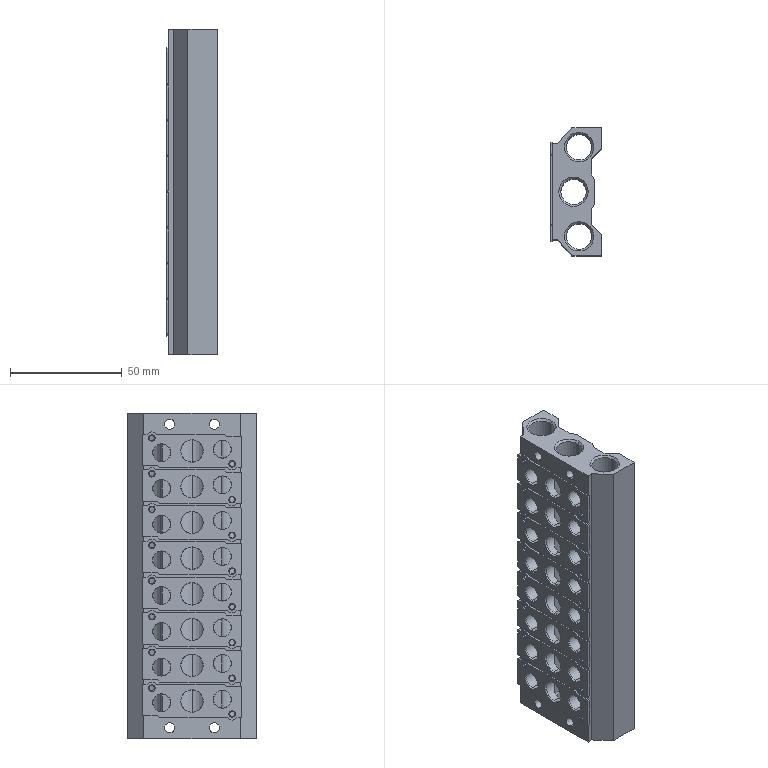Part | STEP file | Solenoid valve base 7V100M8F | 1 solid | 478 faces | box 22.8 x 57.5 x 146 mm | volume 85064 mm3 | cylinder 242 | plane 192 | cone 44 | commonest cylinder face diameters 1 x32 2.459 x32 3 x32 8 x32 8.05 x32 5.4 x24